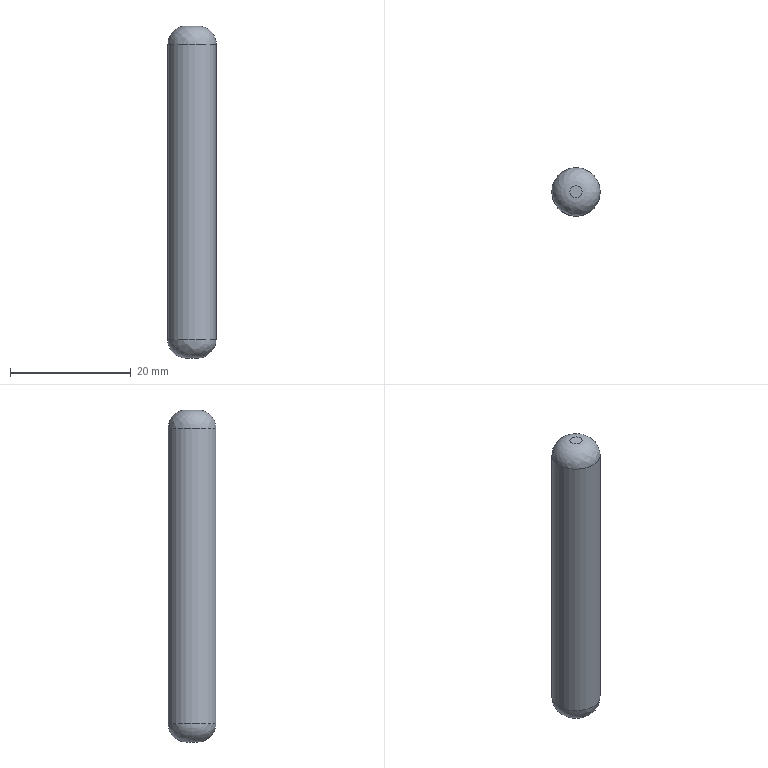Part | STEP file | 1 solid | 5 faces | box 8 x 8 x 55 mm | volume 2684 mm3 | plane 2 | spline 2 | cylinder 1 | commonest cylinder face diameters 8 x1
STEP:
#1=CARTESIAN_POINT('',(0.,0.,0.));
#2=DIRECTION('',(0.,0.,1.));
#3=DIRECTION('',(1.,0.,0.));
#4=AXIS2_PLACEMENT_3D('',#1,#2,#3);
#5=CARTESIAN_POINT('',(1513.247,357.48,-62.381));
#6=VERTEX_POINT('',#5);
#7=CARTESIAN_POINT('',(1512.247,357.48,-62.381));
#8=DIRECTION('',(0.,0.,1.));
#9=DIRECTION('',(1.,0.,0.));
#10=AXIS2_PLACEMENT_3D('',#7,#8,#9);
#11=CIRCLE('',#10,1.);
#12=CARTESIAN_POINT('',(1512.247,357.48,-62.381));
#13=DIRECTION('',(0.,0.,1.));
#14=DIRECTION('',(-1.,0.,0.));
#15=AXIS2_PLACEMENT_3D('',#12,#13,#14);
#16=PLANE('',#15);
#17=CARTESIAN_POINT('',(0.,0.));
#18=DIRECTION('',(-1.,0.));
#19=AXIS2_PLACEMENT_2D('',#17,#18);
#20=CIRCLE('',#19,1.);
#21=(GEOMETRIC_REPRESENTATION_CONTEXT(2)PARAMETRIC_REPRESENTATION_CONTEXT()REPRESENTATION_CONTEXT('',''));
#22=DEFINITIONAL_REPRESENTATION('',(#20),#21);
#23=PCURVE('',#16,#22);
#24=CARTESIAN_POINT('',(1513.247,357.48,-62.381));
#25=CARTESIAN_POINT('',(1513.247,359.48,-62.381));
#26=CARTESIAN_POINT('',(1511.247,359.48,-62.381));
#27=CARTESIAN_POINT('',(1511.247,357.48,-62.381));
#28=CARTESIAN_POINT('',(1511.247,355.48,-62.381));
#29=CARTESIAN_POINT('',(1513.247,355.48,-62.381));
#30=CARTESIAN_POINT('',(1513.247,357.48,-62.381));
#31=CARTESIAN_POINT('',(1515.005,357.48,-62.381));
#32=CARTESIAN_POINT('',(1515.005,362.995,-62.381));
#33=CARTESIAN_POINT('',(1509.49,362.995,-62.381));
#34=CARTESIAN_POINT('',(1509.49,357.48,-62.381));
#35=CARTESIAN_POINT('',(1509.49,351.966,-62.381));
#36=CARTESIAN_POINT('',(1515.005,351.966,-62.381));
#37=CARTESIAN_POINT('',(1515.005,357.48,-62.381));
#38=CARTESIAN_POINT('',(1516.247,357.48,-63.624));
#39=CARTESIAN_POINT('',(1516.247,365.48,-63.624));
#40=CARTESIAN_POINT('',(1508.247,365.48,-63.624));
#41=CARTESIAN_POINT('',(1508.247,357.48,-63.624));
#42=CARTESIAN_POINT('',(1508.247,349.48,-63.624));
#43=CARTESIAN_POINT('',(1516.247,349.48,-63.624));
#44=CARTESIAN_POINT('',(1516.247,357.48,-63.624));
#45=CARTESIAN_POINT('',(1516.247,357.48,-65.381));
#46=CARTESIAN_POINT('',(1516.247,365.48,-65.381));
#47=CARTESIAN_POINT('',(1508.247,365.48,-65.381));
#48=CARTESIAN_POINT('',(1508.247,357.48,-65.381));
#49=CARTESIAN_POINT('',(1508.247,349.48,-65.381));
#50=CARTESIAN_POINT('',(1516.247,349.48,-65.381));
#51=CARTESIAN_POINT('',(1516.247,357.48,-65.381));
#52=(BOUNDED_SURFACE()B_SPLINE_SURFACE(3,3,((#24,#25,#26,#27,#28,#29,#30),(#31,#32,#33,#34,#35,#36,#37),(#38,#39,#40,#41,#42,#43,#44),(#45,#46,#47,#48,#49,#50,#51)),.UNSPECIFIED.,.F.,.T.,.F.)B_SPLINE_SURFACE_WITH_KNOTS((4,4),(1,3,3,3,1),(0.,1.),(-0.5,0.,0.5,1.,1.5),.UNSPECIFIED.)GEOMETRIC_REPRESENTATION_ITEM()RATIONAL_B_SPLINE_SURFACE(((1.,0.3333,0.3333,1.,0.3333,0.3333,1.),(0.8047,0.2682,0.2682,0.8047,0.2682,0.2682,0.8047),(0.8047,0.2682,0.2682,0.8047,0.2682,0.2682,0.8047),(1.,0.3333,0.3333,1.,0.3333,0.3333,1.)))REPRESENTATION_ITEM('')SURFACE());
#53=CARTESIAN_POINT('',(0.,0.));
#54=CARTESIAN_POINT('',(0.,0.02352));
#55=CARTESIAN_POINT('',(0.,0.06491));
#56=CARTESIAN_POINT('',(0.,0.1146));
#57=CARTESIAN_POINT('',(0.,0.1575));
#58=CARTESIAN_POINT('',(0.,0.196));
#59=CARTESIAN_POINT('',(0.,0.2322));
#60=CARTESIAN_POINT('',(0.,0.2678));
#61=CARTESIAN_POINT('',(0.,0.304));
#62=CARTESIAN_POINT('',(0.,0.3425));
#63=CARTESIAN_POINT('',(0.,0.3856));
#64=CARTESIAN_POINT('',(0.,0.4343));
#65=CARTESIAN_POINT('',(0.,0.5));
#66=CARTESIAN_POINT('',(0.,0.5657));
#67=CARTESIAN_POINT('',(0.,0.6144));
#68=CARTESIAN_POINT('',(0.,0.6575));
#69=CARTESIAN_POINT('',(0.,0.696));
#70=CARTESIAN_POINT('',(0.,0.7322));
#71=CARTESIAN_POINT('',(0.,0.7678));
#72=CARTESIAN_POINT('',(0.,0.804));
#73=CARTESIAN_POINT('',(0.,0.8425));
#74=CARTESIAN_POINT('',(0.,0.8854));
#75=CARTESIAN_POINT('',(0.,0.9351));
#76=CARTESIAN_POINT('',(0.,0.9765));
#77=CARTESIAN_POINT('',(0.,1.));
#78=B_SPLINE_CURVE_WITH_KNOTS('',3,(#53,#54,#55,#56,#57,#58,#59,#60,#61,#62,#63,#64,#65,#66,#67,#68,#69,#70,#71,#72,#73,#74,#75,#76,#77),.UNSPECIFIED.,.F.,.F.,(4,1,1,1,1,1,1,1,1,1,1,1,1,1,1,1,1,1,1,1,1,1,4),(0.,0.2856,0.5712,0.8568,1.142,1.428,1.714,1.999,2.285,2.57,2.856,3.142,3.427,3.713,3.998,4.284,4.57,4.855,5.141,5.426,5.712,5.998,6.283),.QUASI_UNIFORM_KNOTS.);
#79=(GEOMETRIC_REPRESENTATION_CONTEXT(2)PARAMETRIC_REPRESENTATION_CONTEXT()REPRESENTATION_CONTEXT('',''));
#80=DEFINITIONAL_REPRESENTATION('',(#78),#79);
#81=PCURVE('',#52,#80);
#82=SURFACE_CURVE('',#11,(#23,#81),.PCURVE_S1.);
#83=EDGE_CURVE('',#6,#6,#82,.T.);
#84=ORIENTED_EDGE('',*,*,#83,.T.);
#85=EDGE_LOOP('',(#84));
#86=FACE_BOUND('',#85,.T.);
#87=ADVANCED_FACE('',(#86),#16,.T.);
#88=CARTESIAN_POINT('',(1511.247,357.48,-117.381));
#89=VERTEX_POINT('',#88);
#90=CARTESIAN_POINT('',(1512.247,357.48,-117.381));
#91=DIRECTION('',(0.,0.,-1.));
#92=DIRECTION('',(-1.,0.,0.));
#93=AXIS2_PLACEMENT_3D('',#90,#91,#92);
#94=CIRCLE('',#93,1.);
#95=CARTESIAN_POINT('',(1512.247,357.48,-117.381));
#96=DIRECTION('',(0.,0.,-1.));
#97=DIRECTION('',(1.,0.,0.));
#98=AXIS2_PLACEMENT_3D('',#95,#96,#97);
#99=PLANE('',#98);
#100=CARTESIAN_POINT('',(0.,0.));
#101=DIRECTION('',(-1.,0.));
#102=AXIS2_PLACEMENT_2D('',#100,#101);
#103=CIRCLE('',#102,1.);
#104=(GEOMETRIC_REPRESENTATION_CONTEXT(2)PARAMETRIC_REPRESENTATION_CONTEXT()REPRESENTATION_CONTEXT('',''));
#105=DEFINITIONAL_REPRESENTATION('',(#103),#104);
#106=PCURVE('',#99,#105);
#107=CARTESIAN_POINT('',(1512.247,358.48,-117.381));
#108=CARTESIAN_POINT('',(1514.247,358.48,-117.381));
#109=CARTESIAN_POINT('',(1514.247,356.48,-117.381));
#110=CARTESIAN_POINT('',(1512.247,356.48,-117.381));
#111=CARTESIAN_POINT('',(1510.247,356.48,-117.381));
#112=CARTESIAN_POINT('',(1510.247,358.48,-117.381));
#113=CARTESIAN_POINT('',(1512.247,358.48,-117.381));
#114=CARTESIAN_POINT('',(1512.247,360.238,-117.381));
#115=CARTESIAN_POINT('',(1517.762,360.238,-117.381));
#116=CARTESIAN_POINT('',(1517.762,354.723,-117.381));
#117=CARTESIAN_POINT('',(1512.247,354.723,-117.381));
#118=CARTESIAN_POINT('',(1506.732,354.723,-117.381));
#119=CARTESIAN_POINT('',(1506.732,360.238,-117.381));
#120=CARTESIAN_POINT('',(1512.247,360.238,-117.381));
#121=CARTESIAN_POINT('',(1512.247,361.48,-116.138));
#122=CARTESIAN_POINT('',(1520.247,361.48,-116.138));
#123=CARTESIAN_POINT('',(1520.247,353.48,-116.138));
#124=CARTESIAN_POINT('',(1512.247,353.48,-116.138));
#125=CARTESIAN_POINT('',(1504.247,353.48,-116.138));
#126=CARTESIAN_POINT('',(1504.247,361.48,-116.138));
#127=CARTESIAN_POINT('',(1512.247,361.48,-116.138));
#128=CARTESIAN_POINT('',(1512.247,361.48,-114.381));
#129=CARTESIAN_POINT('',(1520.247,361.48,-114.381));
#130=CARTESIAN_POINT('',(1520.247,353.48,-114.381));
#131=CARTESIAN_POINT('',(1512.247,353.48,-114.381));
#132=CARTESIAN_POINT('',(1504.247,353.48,-114.381));
#133=CARTESIAN_POINT('',(1504.247,361.48,-114.381));
#134=CARTESIAN_POINT('',(1512.247,361.48,-114.381));
#135=(BOUNDED_SURFACE()B_SPLINE_SURFACE(3,3,((#107,#108,#109,#110,#111,#112,#113),(#114,#115,#116,#117,#118,#119,#120),(#121,#122,#123,#124,#125,#126,#127),(#128,#129,#130,#131,#132,#133,#134)),.UNSPECIFIED.,.F.,.T.,.F.)B_SPLINE_SURFACE_WITH_KNOTS((4,4),(1,3,3,3,1),(0.,1.),(-0.5,0.,0.5,1.,1.5),.UNSPECIFIED.)GEOMETRIC_REPRESENTATION_ITEM()RATIONAL_B_SPLINE_SURFACE(((1.,0.3333,0.3333,1.,0.3333,0.3333,1.),(0.8047,0.2682,0.2682,0.8047,0.2682,0.2682,0.8047),(0.8047,0.2682,0.2682,0.8047,0.2682,0.2682,0.8047),(1.,0.3333,0.3333,1.,0.3333,0.3333,1.)))REPRESENTATION_ITEM('')SURFACE());
#136=CARTESIAN_POINT('',(0.,0.75));
#137=CARTESIAN_POINT('',(0.,0.7619));
#138=CARTESIAN_POINT('',(0.,0.7857));
#139=CARTESIAN_POINT('',(0.,0.8229));
#140=CARTESIAN_POINT('',(0.,0.8632));
#141=CARTESIAN_POINT('',(0.,0.9093));
#142=CARTESIAN_POINT('',(0.,0.9635));
#143=CARTESIAN_POINT('',(0.,1.037));
#144=CARTESIAN_POINT('',(0.,1.091));
#145=CARTESIAN_POINT('',(0.,1.137));
#146=CARTESIAN_POINT('',(0.,1.177));
#147=CARTESIAN_POINT('',(0.,1.214));
#148=CARTESIAN_POINT('',(0.,1.25));
#149=CARTESIAN_POINT('',(0.,1.286));
#150=CARTESIAN_POINT('',(0.,1.323));
#151=CARTESIAN_POINT('',(0.,1.363));
#152=CARTESIAN_POINT('',(0.,1.409));
#153=CARTESIAN_POINT('',(0.,1.463));
#154=CARTESIAN_POINT('',(0.,1.537));
#155=CARTESIAN_POINT('',(0.,1.591));
#156=CARTESIAN_POINT('',(0.,1.637));
#157=CARTESIAN_POINT('',(0.,1.677));
#158=CARTESIAN_POINT('',(0.,1.714));
#159=CARTESIAN_POINT('',(0.,1.738));
#160=CARTESIAN_POINT('',(0.,1.75));
#161=B_SPLINE_CURVE_WITH_KNOTS('',3,(#136,#137,#138,#139,#140,#141,#142,#143,#144,#145,#146,#147,#148,#149,#150,#151,#152,#153,#154,#155,#156,#157,#158,#159,#160),.UNSPECIFIED.,.F.,.F.,(4,1,1,1,1,1,1,1,1,1,1,1,1,1,1,1,1,1,1,1,1,1,4),(0.,0.2856,0.5712,0.8568,1.142,1.428,1.714,1.999,2.285,2.57,2.856,3.142,3.427,3.713,3.998,4.284,4.57,4.855,5.141,5.426,5.712,5.998,6.283),.QUASI_UNIFORM_KNOTS.);
#162=(GEOMETRIC_REPRESENTATION_CONTEXT(2)PARAMETRIC_REPRESENTATION_CONTEXT()REPRESENTATION_CONTEXT('',''));
#163=DEFINITIONAL_REPRESENTATION('',(#161),#162);
#164=PCURVE('',#135,#163);
#165=SURFACE_CURVE('',#94,(#106,#164),.PCURVE_S1.);
#166=EDGE_CURVE('',#89,#89,#165,.T.);
#167=ORIENTED_EDGE('',*,*,#166,.T.);
#168=EDGE_LOOP('',(#167));
#169=FACE_BOUND('',#168,.T.);
#170=ADVANCED_FACE('',(#169),#99,.T.);
#171=CARTESIAN_POINT('',(1508.247,357.48,-114.381));
#172=VERTEX_POINT('',#171);
#173=CARTESIAN_POINT('',(1512.247,357.48,-114.381));
#174=DIRECTION('',(0.,0.,1.));
#175=DIRECTION('',(-1.,0.,0.));
#176=AXIS2_PLACEMENT_3D('',#173,#174,#175);
#177=CIRCLE('',#176,4.);
#178=CARTESIAN_POINT('',(1512.247,357.48,-87.381));
#179=DIRECTION('',(0.,0.,1.));
#180=DIRECTION('',(-1.,0.,0.));
#181=AXIS2_PLACEMENT_3D('',#178,#179,#180);
#182=CYLINDRICAL_SURFACE('',#181,4.);
#183=CARTESIAN_POINT('',(0.,-27.));
#184=DIRECTION('',(1.,0.));
#185=VECTOR('',#184,1.);
#186=LINE('',#183,#185);
#187=(GEOMETRIC_REPRESENTATION_CONTEXT(2)PARAMETRIC_REPRESENTATION_CONTEXT()REPRESENTATION_CONTEXT('',''));
#188=DEFINITIONAL_REPRESENTATION('',(#186),#187);
#189=PCURVE('',#182,#188);
#190=CARTESIAN_POINT('',(1.,1.75));
#191=CARTESIAN_POINT('',(1.,1.738));
#192=CARTESIAN_POINT('',(1.,1.714));
#193=CARTESIAN_POINT('',(1.,1.677));
#194=CARTESIAN_POINT('',(1.,1.637));
#195=CARTESIAN_POINT('',(1.,1.591));
#196=CARTESIAN_POINT('',(1.,1.537));
#197=CARTESIAN_POINT('',(1.,1.463));
#198=CARTESIAN_POINT('',(1.,1.409));
#199=CARTESIAN_POINT('',(1.,1.363));
#200=CARTESIAN_POINT('',(1.,1.323));
#201=CARTESIAN_POINT('',(1.,1.286));
#202=CARTESIAN_POINT('',(1.,1.25));
#203=CARTESIAN_POINT('',(1.,1.214));
#204=CARTESIAN_POINT('',(1.,1.177));
#205=CARTESIAN_POINT('',(1.,1.137));
#206=CARTESIAN_POINT('',(1.,1.091));
#207=CARTESIAN_POINT('',(1.,1.037));
#208=CARTESIAN_POINT('',(1.,0.9635));
#209=CARTESIAN_POINT('',(1.,0.9093));
#210=CARTESIAN_POINT('',(1.,0.8632));
#211=CARTESIAN_POINT('',(1.,0.8229));
#212=CARTESIAN_POINT('',(1.,0.7857));
#213=CARTESIAN_POINT('',(1.,0.7619));
#214=CARTESIAN_POINT('',(1.,0.75));
#215=B_SPLINE_CURVE_WITH_KNOTS('',3,(#190,#191,#192,#193,#194,#195,#196,#197,#198,#199,#200,#201,#202,#203,#204,#205,#206,#207,#208,#209,#210,#211,#212,#213,#214),.UNSPECIFIED.,.F.,.F.,(4,1,1,1,1,1,1,1,1,1,1,1,1,1,1,1,1,1,1,1,1,1,4),(0.,0.2856,0.5712,0.8568,1.142,1.428,1.714,1.999,2.285,2.57,2.856,3.142,3.427,3.713,3.998,4.284,4.57,4.855,5.141,5.426,5.712,5.998,6.283),.QUASI_UNIFORM_KNOTS.);
#216=(GEOMETRIC_REPRESENTATION_CONTEXT(2)PARAMETRIC_REPRESENTATION_CONTEXT()REPRESENTATION_CONTEXT('',''));
#217=DEFINITIONAL_REPRESENTATION('',(#215),#216);
#218=PCURVE('',#135,#217);
#219=SURFACE_CURVE('',#177,(#189,#218),.PCURVE_S1.);
#220=EDGE_CURVE('',#172,#172,#219,.T.);
#221=ORIENTED_EDGE('',*,*,#220,.T.);
#222=CARTESIAN_POINT('',(1508.247,357.48,-65.381));
#223=VERTEX_POINT('',#222);
#224=CARTESIAN_POINT('',(1508.247,357.48,-114.381));
#225=CARTESIAN_POINT('',(1508.247,357.48,-65.381));
#226=B_SPLINE_CURVE_WITH_KNOTS('',1,(#224,#225),.UNSPECIFIED.,.F.,.F.,(2,2),(-27.,22.),.PIECEWISE_BEZIER_KNOTS.);
#227=CARTESIAN_POINT('',(6.283,0.));
#228=DIRECTION('',(0.,1.));
#229=VECTOR('',#228,1.);
#230=LINE('',#227,#229);
#231=(GEOMETRIC_REPRESENTATION_CONTEXT(2)PARAMETRIC_REPRESENTATION_CONTEXT()REPRESENTATION_CONTEXT('',''));
#232=DEFINITIONAL_REPRESENTATION('',(#230),#231);
#233=PCURVE('',#182,#232);
#234=CARTESIAN_POINT('',(0.,0.));
#235=DIRECTION('',(0.,1.));
#236=VECTOR('',#235,1.);
#237=LINE('',#234,#236);
#238=(GEOMETRIC_REPRESENTATION_CONTEXT(2)PARAMETRIC_REPRESENTATION_CONTEXT()REPRESENTATION_CONTEXT('',''));
#239=DEFINITIONAL_REPRESENTATION('',(#237),#238);
#240=PCURVE('',#182,#239);
#241=SEAM_CURVE('',#226,(#233,#240),.PCURVE_S1.);
#242=EDGE_CURVE('',#172,#223,#241,.T.);
#243=ORIENTED_EDGE('',*,*,#242,.T.);
#244=CARTESIAN_POINT('',(1516.247,357.48,-65.381));
#245=VERTEX_POINT('',#244);
#246=CARTESIAN_POINT('',(1512.247,357.48,-65.381));
#247=DIRECTION('',(0.,0.,-1.));
#248=DIRECTION('',(1.,0.,0.));
#249=AXIS2_PLACEMENT_3D('',#246,#247,#248);
#250=CIRCLE('',#249,4.);
#251=CARTESIAN_POINT('',(9.425,22.));
#252=DIRECTION('',(-1.,0.));
#253=VECTOR('',#252,1.);
#254=LINE('',#251,#253);
#255=(GEOMETRIC_REPRESENTATION_CONTEXT(2)PARAMETRIC_REPRESENTATION_CONTEXT()REPRESENTATION_CONTEXT('',''));
#256=DEFINITIONAL_REPRESENTATION('',(#254),#255);
#257=PCURVE('',#182,#256);
#258=CARTESIAN_POINT('',(1.,0.5));
#259=CARTESIAN_POINT('',(1.,0.4881));
#260=CARTESIAN_POINT('',(1.,0.466));
#261=CARTESIAN_POINT('',(1.,0.4367));
#262=CARTESIAN_POINT('',(1.,0.4103));
#263=CARTESIAN_POINT('',(1.,0.3862));
#264=CARTESIAN_POINT('',(1.,0.3639));
#265=CARTESIAN_POINT('',(1.,0.3431));
#266=CARTESIAN_POINT('',(1.,0.3233));
#267=CARTESIAN_POINT('',(1.,0.3043));
#268=CARTESIAN_POINT('',(1.,0.2859));
#269=CARTESIAN_POINT('',(1.,0.2678));
#270=CARTESIAN_POINT('',(1.,0.25));
#271=CARTESIAN_POINT('',(1.,0.2322));
#272=CARTESIAN_POINT('',(1.,0.2141));
#273=CARTESIAN_POINT('',(1.,0.1957));
#274=CARTESIAN_POINT('',(1.,0.1767));
#275=CARTESIAN_POINT('',(1.,0.1569));
#276=CARTESIAN_POINT('',(1.,0.1361));
#277=CARTESIAN_POINT('',(1.,0.1138));
#278=CARTESIAN_POINT('',(1.,0.08972));
#279=CARTESIAN_POINT('',(1.,0.06334));
#280=CARTESIAN_POINT('',(1.,0.03403));
#281=CARTESIAN_POINT('',(1.,0.01187));
#282=CARTESIAN_POINT('',(1.,0.));
#283=B_SPLINE_CURVE_WITH_KNOTS('',3,(#258,#259,#260,#261,#262,#263,#264,#265,#266,#267,#268,#269,#270,#271,#272,#273,#274,#275,#276,#277,#278,#279,#280,#281,#282),.UNSPECIFIED.,.F.,.F.,(4,1,1,1,1,1,1,1,1,1,1,1,1,1,1,1,1,1,1,1,1,1,4),(3.142,3.284,3.427,3.57,3.713,3.856,3.998,4.141,4.284,4.427,4.57,4.712,4.855,4.998,5.141,5.284,5.426,5.569,5.712,5.855,5.998,6.14,6.283),.QUASI_UNIFORM_KNOTS.);
#284=(GEOMETRIC_REPRESENTATION_CONTEXT(2)PARAMETRIC_REPRESENTATION_CONTEXT()REPRESENTATION_CONTEXT('',''));
#285=DEFINITIONAL_REPRESENTATION('',(#283),#284);
#286=PCURVE('',#52,#285);
#287=SURFACE_CURVE('',#250,(#257,#286),.PCURVE_S1.);
#288=EDGE_CURVE('',#223,#245,#287,.T.);
#289=ORIENTED_EDGE('',*,*,#288,.T.);
#290=CARTESIAN_POINT('',(1512.247,357.48,-65.381));
#291=DIRECTION('',(0.,0.,-1.));
#292=DIRECTION('',(1.,0.,0.));
#293=AXIS2_PLACEMENT_3D('',#290,#291,#292);
#294=CIRCLE('',#293,4.);
#295=CARTESIAN_POINT('',(3.142,22.));
#296=DIRECTION('',(-1.,0.));
#297=VECTOR('',#296,1.);
#298=LINE('',#295,#297);
#299=(GEOMETRIC_REPRESENTATION_CONTEXT(2)PARAMETRIC_REPRESENTATION_CONTEXT()REPRESENTATION_CONTEXT('',''));
#300=DEFINITIONAL_REPRESENTATION('',(#298),#299);
#301=PCURVE('',#182,#300);
#302=CARTESIAN_POINT('',(1.,1.));
#303=CARTESIAN_POINT('',(1.,0.9881));
#304=CARTESIAN_POINT('',(1.,0.966));
#305=CARTESIAN_POINT('',(1.,0.9367));
#306=CARTESIAN_POINT('',(1.,0.9103));
#307=CARTESIAN_POINT('',(1.,0.8862));
#308=CARTESIAN_POINT('',(1.,0.8639));
#309=CARTESIAN_POINT('',(1.,0.8431));
#310=CARTESIAN_POINT('',(1.,0.8233));
#311=CARTESIAN_POINT('',(1.,0.8043));
#312=CARTESIAN_POINT('',(1.,0.7859));
#313=CARTESIAN_POINT('',(1.,0.7678));
#314=CARTESIAN_POINT('',(1.,0.75));
#315=CARTESIAN_POINT('',(1.,0.7322));
#316=CARTESIAN_POINT('',(1.,0.7141));
#317=CARTESIAN_POINT('',(1.,0.6957));
#318=CARTESIAN_POINT('',(1.,0.6767));
#319=CARTESIAN_POINT('',(1.,0.6569));
#320=CARTESIAN_POINT('',(1.,0.6361));
#321=CARTESIAN_POINT('',(1.,0.6138));
#322=CARTESIAN_POINT('',(1.,0.5897));
#323=CARTESIAN_POINT('',(1.,0.5633));
#324=CARTESIAN_POINT('',(1.,0.534));
#325=CARTESIAN_POINT('',(1.,0.5119));
#326=CARTESIAN_POINT('',(1.,0.5));
#327=B_SPLINE_CURVE_WITH_KNOTS('',3,(#302,#303,#304,#305,#306,#307,#308,#309,#310,#311,#312,#313,#314,#315,#316,#317,#318,#319,#320,#321,#322,#323,#324,#325,#326),.UNSPECIFIED.,.F.,.F.,(4,1,1,1,1,1,1,1,1,1,1,1,1,1,1,1,1,1,1,1,1,1,4),(0.,0.1428,0.2856,0.4284,0.5712,0.714,0.8568,0.9996,1.142,1.285,1.428,1.571,1.714,1.856,1.999,2.142,2.285,2.428,2.57,2.713,2.856,2.999,3.142),.QUASI_UNIFORM_KNOTS.);
#328=(GEOMETRIC_REPRESENTATION_CONTEXT(2)PARAMETRIC_REPRESENTATION_CONTEXT()REPRESENTATION_CONTEXT('',''));
#329=DEFINITIONAL_REPRESENTATION('',(#327),#328);
#330=PCURVE('',#52,#329);
#331=SURFACE_CURVE('',#294,(#301,#330),.PCURVE_S1.);
#332=EDGE_CURVE('',#245,#223,#331,.T.);
#333=ORIENTED_EDGE('',*,*,#332,.T.);
#334=ORIENTED_EDGE('',*,*,#242,.F.);
#335=EDGE_LOOP('',(#221,#243,#289,#333,#334));
#336=FACE_BOUND('',#335,.T.);
#337=ADVANCED_FACE('',(#336),#182,.T.);
#338=ORIENTED_EDGE('',*,*,#166,.F.);
#339=CARTESIAN_POINT('',(1511.247,357.48,-117.381));
#340=CARTESIAN_POINT('',(1509.49,357.48,-117.381));
#341=CARTESIAN_POINT('',(1508.247,357.48,-116.138));
#342=CARTESIAN_POINT('',(1508.247,357.48,-114.381));
#343=(BOUNDED_CURVE()B_SPLINE_CURVE(3,(#339,#340,#341,#342),.UNSPECIFIED.,.F.,.F.)B_SPLINE_CURVE_WITH_KNOTS((4,4),(0.,1.),.PIECEWISE_BEZIER_KNOTS.)CURVE()GEOMETRIC_REPRESENTATION_ITEM()RATIONAL_B_SPLINE_CURVE((0.5,0.4024,0.4024,0.5))REPRESENTATION_ITEM(''));
#344=CARTESIAN_POINT('',(0.,0.75));
#345=DIRECTION('',(1.,0.));
#346=VECTOR('',#345,1.);
#347=LINE('',#344,#346);
#348=(GEOMETRIC_REPRESENTATION_CONTEXT(2)PARAMETRIC_REPRESENTATION_CONTEXT()REPRESENTATION_CONTEXT('',''));
#349=DEFINITIONAL_REPRESENTATION('',(#347),#348);
#350=PCURVE('',#135,#349);
#351=CARTESIAN_POINT('',(0.,1.75));
#352=DIRECTION('',(1.,0.));
#353=VECTOR('',#352,1.);
#354=LINE('',#351,#353);
#355=(GEOMETRIC_REPRESENTATION_CONTEXT(2)PARAMETRIC_REPRESENTATION_CONTEXT()REPRESENTATION_CONTEXT('',''));
#356=DEFINITIONAL_REPRESENTATION('',(#354),#355);
#357=PCURVE('',#135,#356);
#358=SEAM_CURVE('',#343,(#350,#357),.PCURVE_S1.);
#359=EDGE_CURVE('',#89,#172,#358,.T.);
#360=ORIENTED_EDGE('',*,*,#359,.T.);
#361=ORIENTED_EDGE('',*,*,#220,.F.);
#362=ORIENTED_EDGE('',*,*,#359,.F.);
#363=EDGE_LOOP('',(#338,#360,#361,#362));
#364=FACE_BOUND('',#363,.T.);
#365=ADVANCED_FACE('',(#364),#135,.T.);
#366=ORIENTED_EDGE('',*,*,#83,.F.);
#367=CARTESIAN_POINT('',(1513.247,357.48,-62.381));
#368=CARTESIAN_POINT('',(1515.005,357.48,-62.381));
#369=CARTESIAN_POINT('',(1516.247,357.48,-63.624));
#370=CARTESIAN_POINT('',(1516.247,357.48,-65.381));
#371=(BOUNDED_CURVE()B_SPLINE_CURVE(3,(#367,#368,#369,#370),.UNSPECIFIED.,.F.,.F.)B_SPLINE_CURVE_WITH_KNOTS((4,4),(0.,1.),.PIECEWISE_BEZIER_KNOTS.)CURVE()GEOMETRIC_REPRESENTATION_ITEM()RATIONAL_B_SPLINE_CURVE((1.,0.8047,0.8047,1.))REPRESENTATION_ITEM(''));
#372=CARTESIAN_POINT('',(0.,0.));
#373=DIRECTION('',(1.,0.));
#374=VECTOR('',#373,1.);
#375=LINE('',#372,#374);
#376=(GEOMETRIC_REPRESENTATION_CONTEXT(2)PARAMETRIC_REPRESENTATION_CONTEXT()REPRESENTATION_CONTEXT('',''));
#377=DEFINITIONAL_REPRESENTATION('',(#375),#376);
#378=PCURVE('',#52,#377);
#379=CARTESIAN_POINT('',(0.,1.));
#380=DIRECTION('',(1.,0.));
#381=VECTOR('',#380,1.);
#382=LINE('',#379,#381);
#383=(GEOMETRIC_REPRESENTATION_CONTEXT(2)PARAMETRIC_REPRESENTATION_CONTEXT()REPRESENTATION_CONTEXT('',''));
#384=DEFINITIONAL_REPRESENTATION('',(#382),#383);
#385=PCURVE('',#52,#384);
#386=SEAM_CURVE('',#371,(#378,#385),.PCURVE_S1.);
#387=EDGE_CURVE('',#6,#245,#386,.T.);
#388=ORIENTED_EDGE('',*,*,#387,.T.);
#389=ORIENTED_EDGE('',*,*,#288,.F.);
#390=ORIENTED_EDGE('',*,*,#332,.F.);
#391=ORIENTED_EDGE('',*,*,#387,.F.);
#392=EDGE_LOOP('',(#366,#388,#389,#390,#391));
#393=FACE_BOUND('',#392,.T.);
#394=ADVANCED_FACE('',(#393),#52,.T.);
#395=CLOSED_SHELL('',(#87,#170,#337,#365,#394));
#396=MANIFOLD_SOLID_BREP('',#395);
#397=(LENGTH_UNIT()NAMED_UNIT(*)SI_UNIT(.MILLI.,.METRE.));
#398=UNCERTAINTY_MEASURE_WITH_UNIT(LENGTH_MEASURE(0.00001),#397,'','');
#399=(NAMED_UNIT(*)PLANE_ANGLE_UNIT()SI_UNIT($,.RADIAN.));
#400=(NAMED_UNIT(*)SI_UNIT($,.STERADIAN.)SOLID_ANGLE_UNIT());
#401=(GEOMETRIC_REPRESENTATION_CONTEXT(3)GLOBAL_UNCERTAINTY_ASSIGNED_CONTEXT((#398))GLOBAL_UNIT_ASSIGNED_CONTEXT((#397,#399,#400))REPRESENTATION_CONTEXT('',''));
#402=ADVANCED_BREP_SHAPE_REPRESENTATION('',(#4,#396),#401);